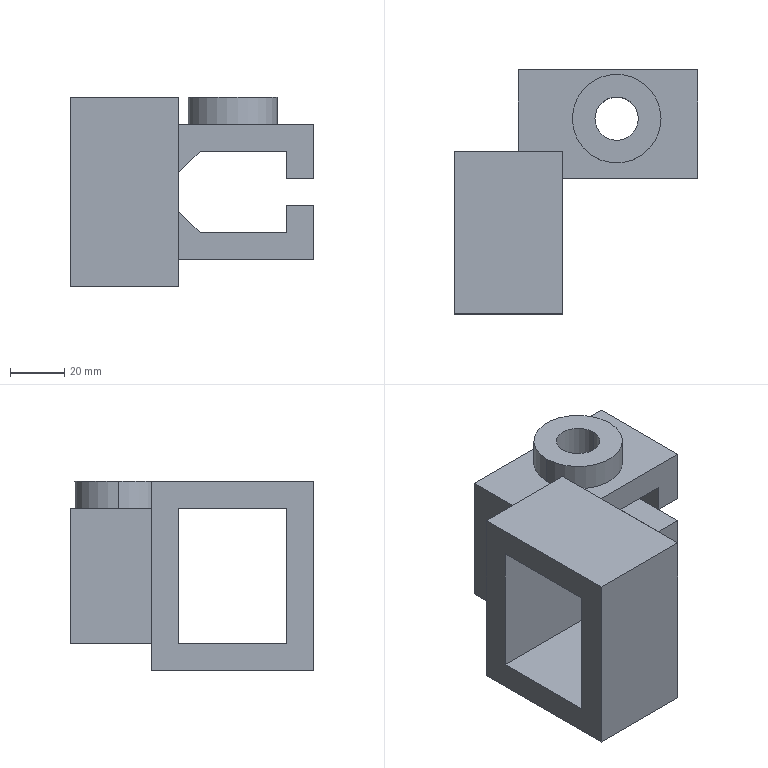Part | SolidWorks | features ICE 5, Extrusion 1 | 1 solid | 32 faces | box 90 x 90 x 70 mm | volume 165265 mm3 | plane 26 | cylinder 6 | commonest cylinder face diameters 16 x4 32.716 x2
STEP:
#1=CARTESIAN_POINT('',(56.358,22.,35.));
#2=VERTEX_POINT('',#1);
#3=CARTESIAN_POINT('',(23.642,22.,35.));
#4=VERTEX_POINT('',#3);
#5=CARTESIAN_POINT('',(40.,22.,35.));
#6=DIRECTION('',(0.,0.,1.));
#7=DIRECTION('',(1.,0.,0.));
#8=AXIS2_PLACEMENT_3D('',#5,#6,#7);
#9=CIRCLE('',#8,16.358);
#10=EDGE_CURVE('',#2,#4,#9,.T.);
#11=ORIENTED_EDGE('',*,*,#10,.F.);
#12=CARTESIAN_POINT('',(56.358,22.,25.));
#13=VERTEX_POINT('',#12);
#14=CARTESIAN_POINT('',(56.358,22.,35.));
#15=DIRECTION('',(0.,0.,-1.));
#16=VECTOR('',#15,1000.);
#17=LINE('',#14,#16);
#18=EDGE_CURVE('',#2,#13,#17,.T.);
#19=ORIENTED_EDGE('',*,*,#18,.T.);
#20=CARTESIAN_POINT('',(23.642,22.,25.));
#21=VERTEX_POINT('',#20);
#22=CARTESIAN_POINT('',(40.,22.,25.));
#23=DIRECTION('',(0.,0.,1.));
#24=DIRECTION('',(-1.,0.,0.));
#25=AXIS2_PLACEMENT_3D('',#22,#23,#24);
#26=CIRCLE('',#25,16.358);
#27=EDGE_CURVE('',#13,#21,#26,.T.);
#28=ORIENTED_EDGE('',*,*,#27,.T.);
#29=CARTESIAN_POINT('',(23.642,22.,35.));
#30=DIRECTION('',(0.,0.,-1.));
#31=VECTOR('',#30,1000.);
#32=LINE('',#29,#31);
#33=EDGE_CURVE('',#4,#21,#32,.T.);
#34=ORIENTED_EDGE('',*,*,#33,.F.);
#35=EDGE_LOOP('',(#11,#19,#28,#34));
#36=FACE_OUTER_BOUND('',#35,.T.);
#37=CARTESIAN_POINT('',(40.,22.,35.));
#38=DIRECTION('',(0.,0.,-1.));
#39=DIRECTION('',(-1.,0.,0.));
#40=AXIS2_PLACEMENT_3D('',#37,#38,#39);
#41=CYLINDRICAL_SURFACE('',#40,16.358);
#42=ADVANCED_FACE('',(#36),#41,.T.);
#43=CARTESIAN_POINT('',(32.,22.,-15.));
#44=VERTEX_POINT('',#43);
#45=CARTESIAN_POINT('',(48.,22.,-15.));
#46=VERTEX_POINT('',#45);
#47=CARTESIAN_POINT('',(40.,22.,-15.));
#48=DIRECTION('',(0.,0.,1.));
#49=DIRECTION('',(1.,0.,0.));
#50=AXIS2_PLACEMENT_3D('',#47,#48,#49);
#51=CIRCLE('',#50,8.);
#52=EDGE_CURVE('',#44,#46,#51,.T.);
#53=ORIENTED_EDGE('',*,*,#52,.T.);
#54=CARTESIAN_POINT('',(48.,22.,-25.));
#55=VERTEX_POINT('',#54);
#56=CARTESIAN_POINT('',(48.,22.,25.));
#57=DIRECTION('',(0.,0.,-1.));
#58=VECTOR('',#57,1000.);
#59=LINE('',#56,#58);
#60=EDGE_CURVE('',#46,#55,#59,.T.);
#61=ORIENTED_EDGE('',*,*,#60,.T.);
#62=CARTESIAN_POINT('',(32.,22.,-25.));
#63=VERTEX_POINT('',#62);
#64=CARTESIAN_POINT('',(40.,22.,-25.));
#65=DIRECTION('',(0.,0.,-1.));
#66=DIRECTION('',(-1.,0.,0.));
#67=AXIS2_PLACEMENT_3D('',#64,#65,#66);
#68=CIRCLE('',#67,8.);
#69=EDGE_CURVE('',#55,#63,#68,.T.);
#70=ORIENTED_EDGE('',*,*,#69,.T.);
#71=CARTESIAN_POINT('',(32.,22.,25.));
#72=DIRECTION('',(0.,0.,-1.));
#73=VECTOR('',#72,1000.);
#74=LINE('',#71,#73);
#75=EDGE_CURVE('',#44,#63,#74,.T.);
#76=ORIENTED_EDGE('',*,*,#75,.F.);
#77=EDGE_LOOP('',(#53,#61,#70,#76));
#78=FACE_OUTER_BOUND('',#77,.T.);
#79=CARTESIAN_POINT('',(40.,22.,25.));
#80=DIRECTION('',(0.,0.,-1.));
#81=DIRECTION('',(-1.,0.,0.));
#82=AXIS2_PLACEMENT_3D('',#79,#80,#81);
#83=CYLINDRICAL_SURFACE('',#82,8.);
#84=ADVANCED_FACE('',(#78),#83,.F.);
#85=CARTESIAN_POINT('',(32.,22.,35.));
#86=VERTEX_POINT('',#85);
#87=CARTESIAN_POINT('',(48.,22.,35.));
#88=VERTEX_POINT('',#87);
#89=CARTESIAN_POINT('',(40.,22.,35.));
#90=DIRECTION('',(0.,0.,1.));
#91=DIRECTION('',(1.,0.,0.));
#92=AXIS2_PLACEMENT_3D('',#89,#90,#91);
#93=CIRCLE('',#92,8.);
#94=EDGE_CURVE('',#86,#88,#93,.T.);
#95=ORIENTED_EDGE('',*,*,#94,.T.);
#96=CARTESIAN_POINT('',(48.,22.,15.));
#97=VERTEX_POINT('',#96);
#98=CARTESIAN_POINT('',(48.,22.,25.));
#99=DIRECTION('',(0.,0.,-1.));
#100=VECTOR('',#99,1000.);
#101=LINE('',#98,#100);
#102=EDGE_CURVE('',#88,#97,#101,.T.);
#103=ORIENTED_EDGE('',*,*,#102,.T.);
#104=CARTESIAN_POINT('',(32.,22.,15.));
#105=VERTEX_POINT('',#104);
#106=CARTESIAN_POINT('',(40.,22.,15.));
#107=DIRECTION('',(0.,0.,-1.));
#108=DIRECTION('',(-1.,0.,0.));
#109=AXIS2_PLACEMENT_3D('',#106,#107,#108);
#110=CIRCLE('',#109,8.);
#111=EDGE_CURVE('',#97,#105,#110,.T.);
#112=ORIENTED_EDGE('',*,*,#111,.T.);
#113=CARTESIAN_POINT('',(32.,22.,25.));
#114=DIRECTION('',(0.,0.,-1.));
#115=VECTOR('',#114,1000.);
#116=LINE('',#113,#115);
#117=EDGE_CURVE('',#86,#105,#116,.T.);
#118=ORIENTED_EDGE('',*,*,#117,.F.);
#119=EDGE_LOOP('',(#95,#103,#112,#118));
#120=FACE_OUTER_BOUND('',#119,.T.);
#121=CARTESIAN_POINT('',(40.,22.,25.));
#122=DIRECTION('',(0.,0.,-1.));
#123=DIRECTION('',(-1.,0.,0.));
#124=AXIS2_PLACEMENT_3D('',#121,#122,#123);
#125=CYLINDRICAL_SURFACE('',#124,8.);
#126=ADVANCED_FACE('',(#120),#125,.F.);
#127=CARTESIAN_POINT('',(20.,0.,25.));
#128=VERTEX_POINT('',#127);
#129=CARTESIAN_POINT('',(20.,10.,25.));
#130=VERTEX_POINT('',#129);
#131=CARTESIAN_POINT('',(20.,-40.,25.));
#132=DIRECTION('',(0.,1.,0.));
#133=VECTOR('',#132,1000.);
#134=LINE('',#131,#133);
#135=EDGE_CURVE('',#128,#130,#134,.T.);
#136=ORIENTED_EDGE('',*,*,#135,.F.);
#137=CARTESIAN_POINT('',(70.,0.,25.));
#138=VERTEX_POINT('',#137);
#139=CARTESIAN_POINT('',(-20.,0.,25.));
#140=DIRECTION('',(1.,0.,0.));
#141=VECTOR('',#140,1000.);
#142=LINE('',#139,#141);
#143=EDGE_CURVE('',#128,#138,#142,.T.);
#144=ORIENTED_EDGE('',*,*,#143,.T.);
#145=CARTESIAN_POINT('',(70.,40.,25.));
#146=VERTEX_POINT('',#145);
#147=CARTESIAN_POINT('',(70.,0.,25.));
#148=DIRECTION('',(0.,1.,0.));
#149=VECTOR('',#148,1000.);
#150=LINE('',#147,#149);
#151=EDGE_CURVE('',#138,#146,#150,.T.);
#152=ORIENTED_EDGE('',*,*,#151,.T.);
#153=CARTESIAN_POINT('',(3.78,40.,25.));
#154=VERTEX_POINT('',#153);
#155=CARTESIAN_POINT('',(3.78,40.,25.));
#156=DIRECTION('',(1.,0.,0.));
#157=VECTOR('',#156,1000.);
#158=LINE('',#155,#157);
#159=EDGE_CURVE('',#154,#146,#158,.T.);
#160=ORIENTED_EDGE('',*,*,#159,.F.);
#161=CARTESIAN_POINT('',(3.78,10.,25.));
#162=VERTEX_POINT('',#161);
#163=CARTESIAN_POINT('',(3.78,40.,25.));
#164=DIRECTION('',(0.,-1.,0.));
#165=VECTOR('',#164,1000.);
#166=LINE('',#163,#165);
#167=EDGE_CURVE('',#154,#162,#166,.T.);
#168=ORIENTED_EDGE('',*,*,#167,.T.);
#169=CARTESIAN_POINT('',(3.78,10.,25.));
#170=DIRECTION('',(1.,0.,0.));
#171=VECTOR('',#170,1000.);
#172=LINE('',#169,#171);
#173=EDGE_CURVE('',#162,#130,#172,.T.);
#174=ORIENTED_EDGE('',*,*,#173,.T.);
#175=EDGE_LOOP('',(#136,#144,#152,#160,#168,#174));
#176=FACE_OUTER_BOUND('',#175,.T.);
#177=CARTESIAN_POINT('',(40.,22.,25.));
#178=DIRECTION('',(0.,0.,1.));
#179=DIRECTION('',(-1.,0.,0.));
#180=AXIS2_PLACEMENT_3D('',#177,#178,#179);
#181=CIRCLE('',#180,16.358);
#182=EDGE_CURVE('',#21,#13,#181,.T.);
#183=ORIENTED_EDGE('',*,*,#182,.F.);
#184=ORIENTED_EDGE('',*,*,#27,.F.);
#185=EDGE_LOOP('',(#183,#184));
#186=FACE_BOUND('',#185,.T.);
#187=CARTESIAN_POINT('',(-20.,10.,25.));
#188=DIRECTION('',(0.,0.,-1.));
#189=DIRECTION('',(-1.,0.,0.));
#190=AXIS2_PLACEMENT_3D('',#187,#188,#189);
#191=PLANE('',#190);
#192=ADVANCED_FACE('',(#176,#186),#191,.F.);
#193=CARTESIAN_POINT('',(40.,22.,-25.));
#194=DIRECTION('',(0.,0.,-1.));
#195=DIRECTION('',(-1.,0.,0.));
#196=AXIS2_PLACEMENT_3D('',#193,#194,#195);
#197=CIRCLE('',#196,8.);
#198=EDGE_CURVE('',#63,#55,#197,.T.);
#199=ORIENTED_EDGE('',*,*,#198,.F.);
#200=ORIENTED_EDGE('',*,*,#69,.F.);
#201=EDGE_LOOP('',(#199,#200));
#202=FACE_BOUND('',#201,.T.);
#203=CARTESIAN_POINT('',(20.,10.,-25.));
#204=VERTEX_POINT('',#203);
#205=CARTESIAN_POINT('',(20.,0.,-25.));
#206=VERTEX_POINT('',#205);
#207=CARTESIAN_POINT('',(20.,0.,-25.));
#208=DIRECTION('',(0.,-1.,0.));
#209=VECTOR('',#208,1000.);
#210=LINE('',#207,#209);
#211=EDGE_CURVE('',#204,#206,#210,.T.);
#212=ORIENTED_EDGE('',*,*,#211,.F.);
#213=CARTESIAN_POINT('',(3.78,10.,-25.));
#214=VERTEX_POINT('',#213);
#215=CARTESIAN_POINT('',(70.,10.,-25.));
#216=DIRECTION('',(-1.,0.,0.));
#217=VECTOR('',#216,1000.);
#218=LINE('',#215,#217);
#219=EDGE_CURVE('',#204,#214,#218,.T.);
#220=ORIENTED_EDGE('',*,*,#219,.T.);
#221=CARTESIAN_POINT('',(3.78,40.,-25.));
#222=VERTEX_POINT('',#221);
#223=CARTESIAN_POINT('',(3.78,40.,-25.));
#224=DIRECTION('',(0.,-1.,0.));
#225=VECTOR('',#224,1000.);
#226=LINE('',#223,#225);
#227=EDGE_CURVE('',#222,#214,#226,.T.);
#228=ORIENTED_EDGE('',*,*,#227,.F.);
#229=CARTESIAN_POINT('',(70.,40.,-25.));
#230=VERTEX_POINT('',#229);
#231=CARTESIAN_POINT('',(70.,40.,-25.));
#232=DIRECTION('',(-1.,0.,0.));
#233=VECTOR('',#232,1000.);
#234=LINE('',#231,#233);
#235=EDGE_CURVE('',#230,#222,#234,.T.);
#236=ORIENTED_EDGE('',*,*,#235,.F.);
#237=CARTESIAN_POINT('',(70.,0.,-25.));
#238=VERTEX_POINT('',#237);
#239=CARTESIAN_POINT('',(70.,0.,-25.));
#240=DIRECTION('',(0.,1.,0.));
#241=VECTOR('',#240,1000.);
#242=LINE('',#239,#241);
#243=EDGE_CURVE('',#238,#230,#242,.T.);
#244=ORIENTED_EDGE('',*,*,#243,.F.);
#245=CARTESIAN_POINT('',(-20.,0.,-25.));
#246=DIRECTION('',(-1.,0.,0.));
#247=VECTOR('',#246,1000.);
#248=LINE('',#245,#247);
#249=EDGE_CURVE('',#238,#206,#248,.T.);
#250=ORIENTED_EDGE('',*,*,#249,.T.);
#251=EDGE_LOOP('',(#212,#220,#228,#236,#244,#250));
#252=FACE_OUTER_BOUND('',#251,.T.);
#253=CARTESIAN_POINT('',(-20.,10.,-25.));
#254=DIRECTION('',(0.,0.,1.));
#255=DIRECTION('',(1.,0.,0.));
#256=AXIS2_PLACEMENT_3D('',#253,#254,#255);
#257=PLANE('',#256);
#258=ADVANCED_FACE('',(#202,#252),#257,.F.);
#259=CARTESIAN_POINT('',(20.,0.,7.));
#260=VERTEX_POINT('',#259);
#261=CARTESIAN_POINT('',(20.,40.,7.));
#262=VERTEX_POINT('',#261);
#263=CARTESIAN_POINT('',(20.,0.,7.));
#264=DIRECTION('',(0.,1.,0.));
#265=VECTOR('',#264,1000.);
#266=LINE('',#263,#265);
#267=EDGE_CURVE('',#260,#262,#266,.T.);
#268=ORIENTED_EDGE('',*,*,#267,.F.);
#269=CARTESIAN_POINT('',(20.,0.,-7.));
#270=VERTEX_POINT('',#269);
#271=CARTESIAN_POINT('',(20.,0.,-25.));
#272=DIRECTION('',(0.,0.,-1.));
#273=VECTOR('',#272,1000.);
#274=LINE('',#271,#273);
#275=EDGE_CURVE('',#260,#270,#274,.T.);
#276=ORIENTED_EDGE('',*,*,#275,.T.);
#277=CARTESIAN_POINT('',(20.,40.,-7.));
#278=VERTEX_POINT('',#277);
#279=CARTESIAN_POINT('',(20.,0.,-7.));
#280=DIRECTION('',(0.,1.,0.));
#281=VECTOR('',#280,1000.);
#282=LINE('',#279,#281);
#283=EDGE_CURVE('',#270,#278,#282,.T.);
#284=ORIENTED_EDGE('',*,*,#283,.T.);
#285=CARTESIAN_POINT('',(20.,40.,7.));
#286=DIRECTION('',(0.,0.,-1.));
#287=VECTOR('',#286,1000.);
#288=LINE('',#285,#287);
#289=EDGE_CURVE('',#262,#278,#288,.T.);
#290=ORIENTED_EDGE('',*,*,#289,.F.);
#291=EDGE_LOOP('',(#268,#276,#284,#290));
#292=FACE_OUTER_BOUND('',#291,.T.);
#293=CARTESIAN_POINT('',(20.,10.,-25.));
#294=DIRECTION('',(-1.,0.,0.));
#295=DIRECTION('',(0.,0.,1.));
#296=AXIS2_PLACEMENT_3D('',#293,#294,#295);
#297=PLANE('',#296);
#298=ADVANCED_FACE('',(#292),#297,.F.);
#299=CARTESIAN_POINT('',(-20.,-40.,-25.));
#300=VERTEX_POINT('',#299);
#301=CARTESIAN_POINT('',(-20.,0.,-25.));
#302=VERTEX_POINT('',#301);
#303=CARTESIAN_POINT('',(-20.,0.,-25.));
#304=DIRECTION('',(0.,1.,0.));
#305=VECTOR('',#304,1000.);
#306=LINE('',#303,#305);
#307=EDGE_CURVE('',#300,#302,#306,.T.);
#308=ORIENTED_EDGE('',*,*,#307,.T.);
#309=CARTESIAN_POINT('',(-20.,0.,25.));
#310=VERTEX_POINT('',#309);
#311=CARTESIAN_POINT('',(-20.,0.,-25.));
#312=DIRECTION('',(0.,0.,1.));
#313=VECTOR('',#312,1000.);
#314=LINE('',#311,#313);
#315=EDGE_CURVE('',#302,#310,#314,.T.);
#316=ORIENTED_EDGE('',*,*,#315,.T.);
#317=CARTESIAN_POINT('',(-20.,-40.,25.));
#318=VERTEX_POINT('',#317);
#319=CARTESIAN_POINT('',(-20.,-40.,25.));
#320=DIRECTION('',(0.,-1.,0.));
#321=VECTOR('',#320,1000.);
#322=LINE('',#319,#321);
#323=EDGE_CURVE('',#310,#318,#322,.T.);
#324=ORIENTED_EDGE('',*,*,#323,.T.);
#325=CARTESIAN_POINT('',(-20.,-40.,-25.));
#326=DIRECTION('',(0.,0.,-1.));
#327=VECTOR('',#326,1000.);
#328=LINE('',#325,#327);
#329=EDGE_CURVE('',#318,#300,#328,.T.);
#330=ORIENTED_EDGE('',*,*,#329,.T.);
#331=EDGE_LOOP('',(#308,#316,#324,#330));
#332=FACE_BOUND('',#331,.T.);
#333=CARTESIAN_POINT('',(-20.,10.,-35.));
#334=VERTEX_POINT('',#333);
#335=CARTESIAN_POINT('',(-20.,10.,35.));
#336=VERTEX_POINT('',#335);
#337=CARTESIAN_POINT('',(-20.,10.,-25.));
#338=DIRECTION('',(0.,0.,1.));
#339=VECTOR('',#338,1000.);
#340=LINE('',#337,#339);
#341=EDGE_CURVE('',#334,#336,#340,.T.);
#342=ORIENTED_EDGE('',*,*,#341,.F.);
#343=CARTESIAN_POINT('',(-20.,-50.,-35.));
#344=VERTEX_POINT('',#343);
#345=CARTESIAN_POINT('',(-20.,10.,-35.));
#346=DIRECTION('',(0.,-1.,0.));
#347=VECTOR('',#346,1000.);
#348=LINE('',#345,#347);
#349=EDGE_CURVE('',#334,#344,#348,.T.);
#350=ORIENTED_EDGE('',*,*,#349,.T.);
#351=CARTESIAN_POINT('',(-20.,-50.,35.));
#352=VERTEX_POINT('',#351);
#353=CARTESIAN_POINT('',(-20.,-50.,-35.));
#354=DIRECTION('',(0.,0.,1.));
#355=VECTOR('',#354,1000.);
#356=LINE('',#353,#355);
#357=EDGE_CURVE('',#344,#352,#356,.T.);
#358=ORIENTED_EDGE('',*,*,#357,.T.);
#359=CARTESIAN_POINT('',(-20.,-50.,35.));
#360=DIRECTION('',(0.,1.,0.));
#361=VECTOR('',#360,1000.);
#362=LINE('',#359,#361);
#363=EDGE_CURVE('',#352,#336,#362,.T.);
#364=ORIENTED_EDGE('',*,*,#363,.T.);
#365=EDGE_LOOP('',(#342,#350,#358,#364));
#366=FACE_OUTER_BOUND('',#365,.T.);
#367=CARTESIAN_POINT('',(-20.,10.,-25.));
#368=DIRECTION('',(1.,0.,0.));
#369=DIRECTION('',(0.,0.,-1.));
#370=AXIS2_PLACEMENT_3D('',#367,#368,#369);
#371=PLANE('',#370);
#372=ADVANCED_FACE('',(#332,#366),#371,.F.);
#373=ORIENTED_EDGE('',*,*,#173,.F.);
#374=CARTESIAN_POINT('',(3.78,10.,-25.));
#375=DIRECTION('',(0.,0.,1.));
#376=VECTOR('',#375,1000.);
#377=LINE('',#374,#376);
#378=EDGE_CURVE('',#214,#162,#377,.T.);
#379=ORIENTED_EDGE('',*,*,#378,.F.);
#380=ORIENTED_EDGE('',*,*,#219,.F.);
#381=CARTESIAN_POINT('',(20.,10.,-35.));
#382=VERTEX_POINT('',#381);
#383=CARTESIAN_POINT('',(20.,10.,-25.));
#384=DIRECTION('',(0.,0.,1.));
#385=VECTOR('',#384,1000.);
#386=LINE('',#383,#385);
#387=EDGE_CURVE('',#382,#204,#386,.T.);
#388=ORIENTED_EDGE('',*,*,#387,.F.);
#389=CARTESIAN_POINT('',(112.195,10.,-35.));
#390=DIRECTION('',(-1.,0.,0.));
#391=VECTOR('',#390,1000.);
#392=LINE('',#389,#391);
#393=EDGE_CURVE('',#382,#334,#392,.T.);
#394=ORIENTED_EDGE('',*,*,#393,.T.);
#395=ORIENTED_EDGE('',*,*,#341,.T.);
#396=CARTESIAN_POINT('',(20.,10.,35.));
#397=VERTEX_POINT('',#396);
#398=CARTESIAN_POINT('',(112.195,10.,35.));
#399=DIRECTION('',(-1.,0.,0.));
#400=VECTOR('',#399,1000.);
#401=LINE('',#398,#400);
#402=EDGE_CURVE('',#397,#336,#401,.T.);
#403=ORIENTED_EDGE('',*,*,#402,.F.);
#404=CARTESIAN_POINT('',(20.,10.,35.));
#405=DIRECTION('',(0.,0.,1.));
#406=VECTOR('',#405,1000.);
#407=LINE('',#404,#406);
#408=EDGE_CURVE('',#130,#397,#407,.T.);
#409=ORIENTED_EDGE('',*,*,#408,.F.);
#410=EDGE_LOOP('',(#373,#379,#380,#388,#394,#395,#403,#409));
#411=FACE_OUTER_BOUND('',#410,.T.);
#412=CARTESIAN_POINT('',(0.,10.,0.));
#413=DIRECTION('',(0.,1.,0.));
#414=DIRECTION('',(0.,0.,1.));
#415=AXIS2_PLACEMENT_3D('',#412,#413,#414);
#416=PLANE('',#415);
#417=ADVANCED_FACE('',(#411),#416,.T.);
#418=ORIENTED_EDGE('',*,*,#275,.F.);
#419=CARTESIAN_POINT('',(28.,0.,15.));
#420=VERTEX_POINT('',#419);
#421=CARTESIAN_POINT('',(28.,0.,15.));
#422=DIRECTION('',(-0.7071,0.,-0.7071));
#423=VECTOR('',#422,1000.);
#424=LINE('',#421,#423);
#425=EDGE_CURVE('',#420,#260,#424,.T.);
#426=ORIENTED_EDGE('',*,*,#425,.F.);
#427=CARTESIAN_POINT('',(60.,0.,15.));
#428=VERTEX_POINT('',#427);
#429=CARTESIAN_POINT('',(28.,0.,15.));
#430=DIRECTION('',(-1.,0.,0.));
#431=VECTOR('',#430,1000.);
#432=LINE('',#429,#431);
#433=EDGE_CURVE('',#428,#420,#432,.T.);
#434=ORIENTED_EDGE('',*,*,#433,.F.);
#435=CARTESIAN_POINT('',(60.,0.,5.));
#436=VERTEX_POINT('',#435);
#437=CARTESIAN_POINT('',(60.,0.,15.));
#438=DIRECTION('',(0.,0.,1.));
#439=VECTOR('',#438,1000.);
#440=LINE('',#437,#439);
#441=EDGE_CURVE('',#436,#428,#440,.T.);
#442=ORIENTED_EDGE('',*,*,#441,.F.);
#443=CARTESIAN_POINT('',(70.,0.,5.));
#444=VERTEX_POINT('',#443);
#445=CARTESIAN_POINT('',(60.,0.,5.));
#446=DIRECTION('',(-1.,0.,0.));
#447=VECTOR('',#446,1000.);
#448=LINE('',#445,#447);
#449=EDGE_CURVE('',#444,#436,#448,.T.);
#450=ORIENTED_EDGE('',*,*,#449,.F.);
#451=CARTESIAN_POINT('',(70.,0.,5.));
#452=DIRECTION('',(0.,0.,-1.));
#453=VECTOR('',#452,1000.);
#454=LINE('',#451,#453);
#455=EDGE_CURVE('',#138,#444,#454,.T.);
#456=ORIENTED_EDGE('',*,*,#455,.F.);
#457=ORIENTED_EDGE('',*,*,#143,.F.);
#458=CARTESIAN_POINT('',(-20.,0.,25.));
#459=DIRECTION('',(1.,0.,0.));
#460=VECTOR('',#459,1000.);
#461=LINE('',#458,#460);
#462=EDGE_CURVE('',#310,#128,#461,.T.);
#463=ORIENTED_EDGE('',*,*,#462,.F.);
#464=ORIENTED_EDGE('',*,*,#315,.F.);
#465=CARTESIAN_POINT('',(-20.,0.,-25.));
#466=DIRECTION('',(-1.,0.,0.));
#467=VECTOR('',#466,1000.);
#468=LINE('',#465,#467);
#469=EDGE_CURVE('',#206,#302,#468,.T.);
#470=ORIENTED_EDGE('',*,*,#469,.F.);
#471=ORIENTED_EDGE('',*,*,#249,.F.);
#472=CARTESIAN_POINT('',(70.,0.,-5.));
#473=VERTEX_POINT('',#472);
#474=CARTESIAN_POINT('',(70.,0.,-25.));
#475=DIRECTION('',(0.,0.,-1.));
#476=VECTOR('',#475,1000.);
#477=LINE('',#474,#476);
#478=EDGE_CURVE('',#473,#238,#477,.T.);
#479=ORIENTED_EDGE('',*,*,#478,.F.);
#480=CARTESIAN_POINT('',(60.,0.,-5.));
#481=VERTEX_POINT('',#480);
#482=CARTESIAN_POINT('',(70.,0.,-5.));
#483=DIRECTION('',(1.,0.,0.));
#484=VECTOR('',#483,1000.);
#485=LINE('',#482,#484);
#486=EDGE_CURVE('',#481,#473,#485,.T.);
#487=ORIENTED_EDGE('',*,*,#486,.F.);
#488=CARTESIAN_POINT('',(60.,0.,-15.));
#489=VERTEX_POINT('',#488);
#490=CARTESIAN_POINT('',(60.,0.,-5.));
#491=DIRECTION('',(0.,0.,1.));
#492=VECTOR('',#491,1000.);
#493=LINE('',#490,#492);
#494=EDGE_CURVE('',#489,#481,#493,.T.);
#495=ORIENTED_EDGE('',*,*,#494,.F.);
#496=CARTESIAN_POINT('',(28.,0.,-15.));
#497=VERTEX_POINT('',#496);
#498=CARTESIAN_POINT('',(60.,0.,-15.));
#499=DIRECTION('',(1.,0.,0.));
#500=VECTOR('',#499,1000.);
#501=LINE('',#498,#500);
#502=EDGE_CURVE('',#497,#489,#501,.T.);
#503=ORIENTED_EDGE('',*,*,#502,.F.);
#504=CARTESIAN_POINT('',(28.,0.,-15.));
#505=DIRECTION('',(0.7071,0.,-0.7071));
#506=VECTOR('',#505,1000.);
#507=LINE('',#504,#506);
#508=EDGE_CURVE('',#270,#497,#507,.T.);
#509=ORIENTED_EDGE('',*,*,#508,.F.);
#510=EDGE_LOOP('',(#418,#426,#434,#442,#450,#456,#457,#463,#464,#470,#471,#479,#487,#495,#503,#509));
#511=FACE_OUTER_BOUND('',#510,.T.);
#512=CARTESIAN_POINT('',(0.,0.,0.));
#513=DIRECTION('',(0.,1.,0.));
#514=DIRECTION('',(0.,0.,1.));
#515=AXIS2_PLACEMENT_3D('',#512,#513,#514);
#516=PLANE('',#515);
#517=ADVANCED_FACE('',(#511),#516,.F.);
#518=ORIENTED_EDGE('',*,*,#243,.T.);
#519=CARTESIAN_POINT('',(70.,40.,-5.));
#520=VERTEX_POINT('',#519);
#521=CARTESIAN_POINT('',(70.,40.,-5.));
#522=DIRECTION('',(0.,0.,-1.));
#523=VECTOR('',#522,1000.);
#524=LINE('',#521,#523);
#525=EDGE_CURVE('',#520,#230,#524,.T.);
#526=ORIENTED_EDGE('',*,*,#525,.F.);
#527=CARTESIAN_POINT('',(70.,0.,-5.));
#528=DIRECTION('',(0.,1.,0.));
#529=VECTOR('',#528,1000.);
#530=LINE('',#527,#529);
#531=EDGE_CURVE('',#473,#520,#530,.T.);
#532=ORIENTED_EDGE('',*,*,#531,.F.);
#533=ORIENTED_EDGE('',*,*,#478,.T.);
#534=EDGE_LOOP('',(#518,#526,#532,#533));
#535=FACE_OUTER_BOUND('',#534,.T.);
#536=CARTESIAN_POINT('',(70.,0.,-25.));
#537=DIRECTION('',(1.,0.,0.));
#538=DIRECTION('',(0.,0.,-1.));
#539=AXIS2_PLACEMENT_3D('',#536,#537,#538);
#540=PLANE('',#539);
#541=ADVANCED_FACE('',(#535),#540,.T.);
#542=ORIENTED_EDGE('',*,*,#531,.T.);
#543=CARTESIAN_POINT('',(60.,40.,-5.));
#544=VERTEX_POINT('',#543);
#545=CARTESIAN_POINT('',(60.,40.,-5.));
#546=DIRECTION('',(1.,0.,0.));
#547=VECTOR('',#546,1000.);
#548=LINE('',#545,#547);
#549=EDGE_CURVE('',#544,#520,#548,.T.);
#550=ORIENTED_EDGE('',*,*,#549,.F.);
#551=CARTESIAN_POINT('',(60.,0.,-5.));
#552=DIRECTION('',(0.,1.,0.));
#553=VECTOR('',#552,1000.);
#554=LINE('',#551,#553);
#555=EDGE_CURVE('',#481,#544,#554,.T.);
#556=ORIENTED_EDGE('',*,*,#555,.F.);
#557=ORIENTED_EDGE('',*,*,#486,.T.);
#558=EDGE_LOOP('',(#542,#550,#556,#557));
#559=FACE_OUTER_BOUND('',#558,.T.);
#560=CARTESIAN_POINT('',(70.,0.,-5.));
#561=DIRECTION('',(0.,0.,1.));
#562=DIRECTION('',(1.,0.,0.));
#563=AXIS2_PLACEMENT_3D('',#560,#561,#562);
#564=PLANE('',#563);
#565=ADVANCED_FACE('',(#559),#564,.T.);
#566=ORIENTED_EDGE('',*,*,#555,.T.);
#567=CARTESIAN_POINT('',(60.,40.,-15.));
#568=VERTEX_POINT('',#567);
#569=CARTESIAN_POINT('',(60.,40.,-15.));
#570=DIRECTION('',(0.,0.,1.));
#571=VECTOR('',#570,1000.);
#572=LINE('',#569,#571);
#573=EDGE_CURVE('',#568,#544,#572,.T.);
#574=ORIENTED_EDGE('',*,*,#573,.F.);
#575=CARTESIAN_POINT('',(60.,0.,-15.));
#576=DIRECTION('',(0.,1.,0.));
#577=VECTOR('',#576,1000.);
#578=LINE('',#575,#577);
#579=EDGE_CURVE('',#489,#568,#578,.T.);
#580=ORIENTED_EDGE('',*,*,#579,.F.);
#581=ORIENTED_EDGE('',*,*,#494,.T.);
#582=EDGE_LOOP('',(#566,#574,#580,#581));
#583=FACE_OUTER_BOUND('',#582,.T.);
#584=CARTESIAN_POINT('',(60.,0.,-5.));
#585=DIRECTION('',(-1.,0.,0.));
#586=DIRECTION('',(0.,0.,1.));
#587=AXIS2_PLACEMENT_3D('',#584,#585,#586);
#588=PLANE('',#587);
#589=ADVANCED_FACE('',(#583),#588,.T.);
#590=ORIENTED_EDGE('',*,*,#52,.F.);
#591=CARTESIAN_POINT('',(40.,22.,-15.));
#592=DIRECTION('',(0.,0.,1.));
#593=DIRECTION('',(1.,0.,0.));
#594=AXIS2_PLACEMENT_3D('',#591,#592,#593);
#595=CIRCLE('',#594,8.);
#596=EDGE_CURVE('',#46,#44,#595,.T.);
#597=ORIENTED_EDGE('',*,*,#596,.F.);
#598=EDGE_LOOP('',(#590,#597));
#599=FACE_BOUND('',#598,.T.);
#600=ORIENTED_EDGE('',*,*,#579,.T.);
#601=CARTESIAN_POINT('',(28.,40.,-15.));
#602=VERTEX_POINT('',#601);
#603=CARTESIAN_POINT('',(28.,40.,-15.));
#604=DIRECTION('',(1.,0.,0.));
#605=VECTOR('',#604,1000.);
#606=LINE('',#603,#605);
#607=EDGE_CURVE('',#602,#568,#606,.T.);
#608=ORIENTED_EDGE('',*,*,#607,.F.);
#609=CARTESIAN_POINT('',(28.,0.,-15.));
#610=DIRECTION('',(0.,1.,0.));
#611=VECTOR('',#610,1000.);
#612=LINE('',#609,#611);
#613=EDGE_CURVE('',#497,#602,#612,.T.);
#614=ORIENTED_EDGE('',*,*,#613,.F.);
#615=ORIENTED_EDGE('',*,*,#502,.T.);
#616=EDGE_LOOP('',(#600,#608,#614,#615));
#617=FACE_OUTER_BOUND('',#616,.T.);
#618=CARTESIAN_POINT('',(60.,0.,-15.));
#619=DIRECTION('',(0.,0.,1.));
#620=DIRECTION('',(1.,0.,0.));
#621=AXIS2_PLACEMENT_3D('',#618,#619,#620);
#622=PLANE('',#621);
#623=ADVANCED_FACE('',(#599,#617),#622,.T.);
#624=ORIENTED_EDGE('',*,*,#613,.T.);
#625=CARTESIAN_POINT('',(20.,40.,-7.));
#626=DIRECTION('',(0.7071,0.,-0.7071));
#627=VECTOR('',#626,1000.);
#628=LINE('',#625,#627);
#629=EDGE_CURVE('',#278,#602,#628,.T.);
#630=ORIENTED_EDGE('',*,*,#629,.F.);
#631=ORIENTED_EDGE('',*,*,#283,.F.);
#632=ORIENTED_EDGE('',*,*,#508,.T.);
#633=EDGE_LOOP('',(#624,#630,#631,#632));
#634=FACE_OUTER_BOUND('',#633,.T.);
#635=CARTESIAN_POINT('',(28.,0.,-15.));
#636=DIRECTION('',(0.7071,0.,0.7071));
#637=DIRECTION('',(0.7071,0.,-0.7071));
#638=AXIS2_PLACEMENT_3D('',#635,#636,#637);
#639=PLANE('',#638);
#640=ADVANCED_FACE('',(#634),#639,.T.);
#641=ORIENTED_EDGE('',*,*,#267,.T.);
#642=CARTESIAN_POINT('',(28.,40.,15.));
#643=VERTEX_POINT('',#642);
#644=CARTESIAN_POINT('',(28.,40.,15.));
#645=DIRECTION('',(-0.7071,0.,-0.7071));
#646=VECTOR('',#645,1000.);
#647=LINE('',#644,#646);
#648=EDGE_CURVE('',#643,#262,#647,.T.);
#649=ORIENTED_EDGE('',*,*,#648,.F.);
#650=CARTESIAN_POINT('',(28.,0.,15.));
#651=DIRECTION('',(0.,1.,0.));
#652=VECTOR('',#651,1000.);
#653=LINE('',#650,#652);
#654=EDGE_CURVE('',#420,#643,#653,.T.);
#655=ORIENTED_EDGE('',*,*,#654,.F.);
#656=ORIENTED_EDGE('',*,*,#425,.T.);
#657=EDGE_LOOP('',(#641,#649,#655,#656));
#658=FACE_OUTER_BOUND('',#657,.T.);
#659=CARTESIAN_POINT('',(28.,0.,15.));
#660=DIRECTION('',(0.7071,0.,-0.7071));
#661=DIRECTION('',(-0.7071,0.,-0.7071));
#662=AXIS2_PLACEMENT_3D('',#659,#660,#661);
#663=PLANE('',#662);
#664=ADVANCED_FACE('',(#658),#663,.T.);
#665=CARTESIAN_POINT('',(40.,22.,15.));
#666=DIRECTION('',(0.,0.,-1.));
#667=DIRECTION('',(-1.,0.,0.));
#668=AXIS2_PLACEMENT_3D('',#665,#666,#667);
#669=CIRCLE('',#668,8.);
#670=EDGE_CURVE('',#105,#97,#669,.T.);
#671=ORIENTED_EDGE('',*,*,#670,.F.);
#672=ORIENTED_EDGE('',*,*,#111,.F.);
#673=EDGE_LOOP('',(#671,#672));
#674=FACE_BOUND('',#673,.T.);
#675=ORIENTED_EDGE('',*,*,#654,.T.);
#676=CARTESIAN_POINT('',(60.,40.,15.));
#677=VERTEX_POINT('',#676);
#678=CARTESIAN_POINT('',(60.,40.,15.));
#679=DIRECTION('',(-1.,0.,0.));
#680=VECTOR('',#679,1000.);
#681=LINE('',#678,#680);
#682=EDGE_CURVE('',#677,#643,#681,.T.);
#683=ORIENTED_EDGE('',*,*,#682,.F.);
#684=CARTESIAN_POINT('',(60.,0.,15.));
#685=DIRECTION('',(0.,1.,0.));
#686=VECTOR('',#685,1000.);
#687=LINE('',#684,#686);
#688=EDGE_CURVE('',#428,#677,#687,.T.);
#689=ORIENTED_EDGE('',*,*,#688,.F.);
#690=ORIENTED_EDGE('',*,*,#433,.T.);
#691=EDGE_LOOP('',(#675,#683,#689,#690));
#692=FACE_OUTER_BOUND('',#691,.T.);
#693=CARTESIAN_POINT('',(28.,0.,15.));
#694=DIRECTION('',(0.,0.,-1.));
#695=DIRECTION('',(-1.,0.,0.));
#696=AXIS2_PLACEMENT_3D('',#693,#694,#695);
#697=PLANE('',#696);
#698=ADVANCED_FACE('',(#674,#692),#697,.T.);
#699=ORIENTED_EDGE('',*,*,#688,.T.);
#700=CARTESIAN_POINT('',(60.,40.,5.));
#701=VERTEX_POINT('',#700);
#702=CARTESIAN_POINT('',(60.,40.,5.));
#703=DIRECTION('',(0.,0.,1.));
#704=VECTOR('',#703,1000.);
#705=LINE('',#702,#704);
#706=EDGE_CURVE('',#701,#677,#705,.T.);
#707=ORIENTED_EDGE('',*,*,#706,.F.);
#708=CARTESIAN_POINT('',(60.,0.,5.));
#709=DIRECTION('',(0.,1.,0.));
#710=VECTOR('',#709,1000.);
#711=LINE('',#708,#710);
#712=EDGE_CURVE('',#436,#701,#711,.T.);
#713=ORIENTED_EDGE('',*,*,#712,.F.);
#714=ORIENTED_EDGE('',*,*,#441,.T.);
#715=EDGE_LOOP('',(#699,#707,#713,#714));
#716=FACE_OUTER_BOUND('',#715,.T.);
#717=CARTESIAN_POINT('',(60.,0.,15.));
#718=DIRECTION('',(-1.,0.,0.));
#719=DIRECTION('',(0.,0.,1.));
#720=AXIS2_PLACEMENT_3D('',#717,#718,#719);
#721=PLANE('',#720);
#722=ADVANCED_FACE('',(#716),#721,.T.);
#723=ORIENTED_EDGE('',*,*,#712,.T.);
#724=CARTESIAN_POINT('',(70.,40.,5.));
#725=VERTEX_POINT('',#724);
#726=CARTESIAN_POINT('',(70.,40.,5.));
#727=DIRECTION('',(-1.,0.,0.));
#728=VECTOR('',#727,1000.);
#729=LINE('',#726,#728);
#730=EDGE_CURVE('',#725,#701,#729,.T.);
#731=ORIENTED_EDGE('',*,*,#730,.F.);
#732=CARTESIAN_POINT('',(70.,0.,5.));
#733=DIRECTION('',(0.,1.,0.));
#734=VECTOR('',#733,1000.);
#735=LINE('',#732,#734);
#736=EDGE_CURVE('',#444,#725,#735,.T.);
#737=ORIENTED_EDGE('',*,*,#736,.F.);
#738=ORIENTED_EDGE('',*,*,#449,.T.);
#739=EDGE_LOOP('',(#723,#731,#737,#738));
#740=FACE_OUTER_BOUND('',#739,.T.);
#741=CARTESIAN_POINT('',(60.,0.,5.));
#742=DIRECTION('',(0.,0.,-1.));
#743=DIRECTION('',(-1.,0.,0.));
#744=AXIS2_PLACEMENT_3D('',#741,#742,#743);
#745=PLANE('',#744);
#746=ADVANCED_FACE('',(#740),#745,.T.);
#747=ORIENTED_EDGE('',*,*,#736,.T.);
#748=CARTESIAN_POINT('',(70.,40.,25.));
#749=DIRECTION('',(0.,0.,-1.));
#750=VECTOR('',#749,1000.);
#751=LINE('',#748,#750);
#752=EDGE_CURVE('',#146,#725,#751,.T.);
#753=ORIENTED_EDGE('',*,*,#752,.F.);
#754=ORIENTED_EDGE('',*,*,#151,.F.);
#755=ORIENTED_EDGE('',*,*,#455,.T.);
#756=EDGE_LOOP('',(#747,#753,#754,#755));
#757=FACE_OUTER_BOUND('',#756,.T.);
#758=CARTESIAN_POINT('',(70.,0.,5.));
#759=DIRECTION('',(1.,0.,0.));
#760=DIRECTION('',(0.,0.,-1.));
#761=AXIS2_PLACEMENT_3D('',#758,#759,#760);
#762=PLANE('',#761);
#763=ADVANCED_FACE('',(#757),#762,.T.);
#764=ORIENTED_EDGE('',*,*,#469,.T.);
#765=ORIENTED_EDGE('',*,*,#307,.F.);
#766=CARTESIAN_POINT('',(20.,-40.,-25.));
#767=VERTEX_POINT('',#766);
#768=CARTESIAN_POINT('',(112.195,-40.,-25.));
#769=DIRECTION('',(-1.,0.,0.));
#770=VECTOR('',#769,1000.);
#771=LINE('',#768,#770);
#772=EDGE_CURVE('',#767,#300,#771,.T.);
#773=ORIENTED_EDGE('',*,*,#772,.F.);
#774=CARTESIAN_POINT('',(20.,0.,-25.));
#775=DIRECTION('',(0.,-1.,0.));
#776=VECTOR('',#775,1000.);
#777=LINE('',#774,#776);
#778=EDGE_CURVE('',#206,#767,#777,.T.);
#779=ORIENTED_EDGE('',*,*,#778,.F.);
#780=EDGE_LOOP('',(#764,#765,#773,#779));
#781=FACE_OUTER_BOUND('',#780,.T.);
#782=CARTESIAN_POINT('',(112.195,0.,-25.));
#783=DIRECTION('',(0.,0.,1.));
#784=DIRECTION('',(1.,0.,0.));
#785=AXIS2_PLACEMENT_3D('',#782,#783,#784);
#786=PLANE('',#785);
#787=ADVANCED_FACE('',(#781),#786,.T.);
#788=ORIENTED_EDGE('',*,*,#462,.T.);
#789=CARTESIAN_POINT('',(20.,-40.,25.));
#790=VERTEX_POINT('',#789);
#791=CARTESIAN_POINT('',(20.,-40.,25.));
#792=DIRECTION('',(0.,1.,0.));
#793=VECTOR('',#792,1000.);
#794=LINE('',#791,#793);
#795=EDGE_CURVE('',#790,#128,#794,.T.);
#796=ORIENTED_EDGE('',*,*,#795,.F.);
#797=CARTESIAN_POINT('',(112.195,-40.,25.));
#798=DIRECTION('',(-1.,0.,0.));
#799=VECTOR('',#798,1000.);
#800=LINE('',#797,#799);
#801=EDGE_CURVE('',#790,#318,#800,.T.);
#802=ORIENTED_EDGE('',*,*,#801,.T.);
#803=ORIENTED_EDGE('',*,*,#323,.F.);
#804=EDGE_LOOP('',(#788,#796,#802,#803));
#805=FACE_OUTER_BOUND('',#804,.T.);
#806=CARTESIAN_POINT('',(112.195,-40.,25.));
#807=DIRECTION('',(0.,0.,-1.));
#808=DIRECTION('',(-1.,0.,0.));
#809=AXIS2_PLACEMENT_3D('',#806,#807,#808);
#810=PLANE('',#809);
#811=ADVANCED_FACE('',(#805),#810,.T.);
#812=CARTESIAN_POINT('',(20.,-40.,-25.));
#813=DIRECTION('',(0.,0.,1.));
#814=VECTOR('',#813,1000.);
#815=LINE('',#812,#814);
#816=EDGE_CURVE('',#767,#790,#815,.T.);
#817=ORIENTED_EDGE('',*,*,#816,.F.);
#818=ORIENTED_EDGE('',*,*,#772,.T.);
#819=ORIENTED_EDGE('',*,*,#329,.F.);
#820=ORIENTED_EDGE('',*,*,#801,.F.);
#821=EDGE_LOOP('',(#817,#818,#819,#820));
#822=FACE_OUTER_BOUND('',#821,.T.);
#823=CARTESIAN_POINT('',(112.195,-40.,-25.));
#824=DIRECTION('',(0.,1.,0.));
#825=DIRECTION('',(0.,0.,1.));
#826=AXIS2_PLACEMENT_3D('',#823,#824,#825);
#827=PLANE('',#826);
#828=ADVANCED_FACE('',(#822),#827,.T.);
#829=CARTESIAN_POINT('',(20.,-50.,35.));
#830=VERTEX_POINT('',#829);
#831=CARTESIAN_POINT('',(20.,-50.,35.));
#832=DIRECTION('',(0.,-1.,0.));
#833=VECTOR('',#832,1000.);
#834=LINE('',#831,#833);
#835=EDGE_CURVE('',#397,#830,#834,.T.);
#836=ORIENTED_EDGE('',*,*,#835,.F.);
#837=ORIENTED_EDGE('',*,*,#402,.T.);
#838=ORIENTED_EDGE('',*,*,#363,.F.);
#839=CARTESIAN_POINT('',(112.195,-50.,35.));
#840=DIRECTION('',(-1.,0.,0.));
#841=VECTOR('',#840,1000.);
#842=LINE('',#839,#841);
#843=EDGE_CURVE('',#830,#352,#842,.T.);
#844=ORIENTED_EDGE('',*,*,#843,.F.);
#845=EDGE_LOOP('',(#836,#837,#838,#844));
#846=FACE_OUTER_BOUND('',#845,.T.);
#847=CARTESIAN_POINT('',(112.195,-50.,35.));
#848=DIRECTION('',(0.,0.,1.));
#849=DIRECTION('',(1.,0.,0.));
#850=AXIS2_PLACEMENT_3D('',#847,#848,#849);
#851=PLANE('',#850);
#852=ADVANCED_FACE('',(#846),#851,.T.);
#853=CARTESIAN_POINT('',(20.,-50.,-35.));
#854=VERTEX_POINT('',#853);
#855=CARTESIAN_POINT('',(20.,-50.,-35.));
#856=DIRECTION('',(0.,0.,-1.));
#857=VECTOR('',#856,1000.);
#858=LINE('',#855,#857);
#859=EDGE_CURVE('',#830,#854,#858,.T.);
#860=ORIENTED_EDGE('',*,*,#859,.F.);
#861=ORIENTED_EDGE('',*,*,#843,.T.);
#862=ORIENTED_EDGE('',*,*,#357,.F.);
#863=CARTESIAN_POINT('',(112.195,-50.,-35.));
#864=DIRECTION('',(-1.,0.,0.));
#865=VECTOR('',#864,1000.);
#866=LINE('',#863,#865);
#867=EDGE_CURVE('',#854,#344,#866,.T.);
#868=ORIENTED_EDGE('',*,*,#867,.F.);
#869=EDGE_LOOP('',(#860,#861,#862,#868));
#870=FACE_OUTER_BOUND('',#869,.T.);
#871=CARTESIAN_POINT('',(112.195,-50.,-35.));
#872=DIRECTION('',(0.,-1.,0.));
#873=DIRECTION('',(0.,0.,-1.));
#874=AXIS2_PLACEMENT_3D('',#871,#872,#873);
#875=PLANE('',#874);
#876=ADVANCED_FACE('',(#870),#875,.T.);
#877=CARTESIAN_POINT('',(20.,10.,-35.));
#878=DIRECTION('',(0.,1.,0.));
#879=VECTOR('',#878,1000.);
#880=LINE('',#877,#879);
#881=EDGE_CURVE('',#854,#382,#880,.T.);
#882=ORIENTED_EDGE('',*,*,#881,.F.);
#883=ORIENTED_EDGE('',*,*,#867,.T.);
#884=ORIENTED_EDGE('',*,*,#349,.F.);
#885=ORIENTED_EDGE('',*,*,#393,.F.);
#886=EDGE_LOOP('',(#882,#883,#884,#885));
#887=FACE_OUTER_BOUND('',#886,.T.);
#888=CARTESIAN_POINT('',(112.195,10.,-35.));
#889=DIRECTION('',(0.,0.,-1.));
#890=DIRECTION('',(-1.,0.,0.));
#891=AXIS2_PLACEMENT_3D('',#888,#889,#890);
#892=PLANE('',#891);
#893=ADVANCED_FACE('',(#887),#892,.T.);
#894=ORIENTED_EDGE('',*,*,#211,.T.);
#895=ORIENTED_EDGE('',*,*,#778,.T.);
#896=ORIENTED_EDGE('',*,*,#816,.T.);
#897=ORIENTED_EDGE('',*,*,#795,.T.);
#898=ORIENTED_EDGE('',*,*,#135,.T.);
#899=ORIENTED_EDGE('',*,*,#408,.T.);
#900=ORIENTED_EDGE('',*,*,#835,.T.);
#901=ORIENTED_EDGE('',*,*,#859,.T.);
#902=ORIENTED_EDGE('',*,*,#881,.T.);
#903=ORIENTED_EDGE('',*,*,#387,.T.);
#904=EDGE_LOOP('',(#894,#895,#896,#897,#898,#899,#900,#901,#902,#903));
#905=FACE_OUTER_BOUND('',#904,.T.);
#906=CARTESIAN_POINT('',(20.,10.,-25.));
#907=DIRECTION('',(-1.,0.,0.));
#908=DIRECTION('',(0.,0.,1.));
#909=AXIS2_PLACEMENT_3D('',#906,#907,#908);
#910=PLANE('',#909);
#911=ADVANCED_FACE('',(#905),#910,.F.);
#912=ORIENTED_EDGE('',*,*,#378,.T.);
#913=ORIENTED_EDGE('',*,*,#167,.F.);
#914=CARTESIAN_POINT('',(3.78,40.,-25.));
#915=DIRECTION('',(0.,0.,1.));
#916=VECTOR('',#915,1000.);
#917=LINE('',#914,#916);
#918=EDGE_CURVE('',#222,#154,#917,.T.);
#919=ORIENTED_EDGE('',*,*,#918,.F.);
#920=ORIENTED_EDGE('',*,*,#227,.T.);
#921=EDGE_LOOP('',(#912,#913,#919,#920));
#922=FACE_OUTER_BOUND('',#921,.T.);
#923=CARTESIAN_POINT('',(3.78,40.,-25.));
#924=DIRECTION('',(1.,0.,0.));
#925=DIRECTION('',(0.,0.,-1.));
#926=AXIS2_PLACEMENT_3D('',#923,#924,#925);
#927=PLANE('',#926);
#928=ADVANCED_FACE('',(#922),#927,.F.);
#929=ORIENTED_EDGE('',*,*,#289,.T.);
#930=ORIENTED_EDGE('',*,*,#629,.T.);
#931=ORIENTED_EDGE('',*,*,#607,.T.);
#932=ORIENTED_EDGE('',*,*,#573,.T.);
#933=ORIENTED_EDGE('',*,*,#549,.T.);
#934=ORIENTED_EDGE('',*,*,#525,.T.);
#935=ORIENTED_EDGE('',*,*,#235,.T.);
#936=ORIENTED_EDGE('',*,*,#918,.T.);
#937=ORIENTED_EDGE('',*,*,#159,.T.);
#938=ORIENTED_EDGE('',*,*,#752,.T.);
#939=ORIENTED_EDGE('',*,*,#730,.T.);
#940=ORIENTED_EDGE('',*,*,#706,.T.);
#941=ORIENTED_EDGE('',*,*,#682,.T.);
#942=ORIENTED_EDGE('',*,*,#648,.T.);
#943=EDGE_LOOP('',(#929,#930,#931,#932,#933,#934,#935,#936,#937,#938,#939,#940,#941,#942));
#944=FACE_OUTER_BOUND('',#943,.T.);
#945=CARTESIAN_POINT('',(0.,40.,0.));
#946=DIRECTION('',(0.,-1.,0.));
#947=DIRECTION('',(0.,0.,-1.));
#948=AXIS2_PLACEMENT_3D('',#945,#946,#947);
#949=PLANE('',#948);
#950=ADVANCED_FACE('',(#944),#949,.F.);
#951=ORIENTED_EDGE('',*,*,#102,.F.);
#952=CARTESIAN_POINT('',(40.,22.,35.));
#953=DIRECTION('',(0.,0.,1.));
#954=DIRECTION('',(1.,0.,0.));
#955=AXIS2_PLACEMENT_3D('',#952,#953,#954);
#956=CIRCLE('',#955,8.);
#957=EDGE_CURVE('',#88,#86,#956,.T.);
#958=ORIENTED_EDGE('',*,*,#957,.T.);
#959=ORIENTED_EDGE('',*,*,#117,.T.);
#960=ORIENTED_EDGE('',*,*,#670,.T.);
#961=EDGE_LOOP('',(#951,#958,#959,#960));
#962=FACE_OUTER_BOUND('',#961,.T.);
#963=CARTESIAN_POINT('',(40.,22.,25.));
#964=DIRECTION('',(0.,0.,-1.));
#965=DIRECTION('',(-1.,0.,0.));
#966=AXIS2_PLACEMENT_3D('',#963,#964,#965);
#967=CYLINDRICAL_SURFACE('',#966,8.);
#968=ADVANCED_FACE('',(#962),#967,.F.);
#969=ORIENTED_EDGE('',*,*,#60,.F.);
#970=ORIENTED_EDGE('',*,*,#596,.T.);
#971=ORIENTED_EDGE('',*,*,#75,.T.);
#972=ORIENTED_EDGE('',*,*,#198,.T.);
#973=EDGE_LOOP('',(#969,#970,#971,#972));
#974=FACE_OUTER_BOUND('',#973,.T.);
#975=CARTESIAN_POINT('',(40.,22.,25.));
#976=DIRECTION('',(0.,0.,-1.));
#977=DIRECTION('',(-1.,0.,0.));
#978=AXIS2_PLACEMENT_3D('',#975,#976,#977);
#979=CYLINDRICAL_SURFACE('',#978,8.);
#980=ADVANCED_FACE('',(#974),#979,.F.);
#981=CARTESIAN_POINT('',(40.,22.,35.));
#982=DIRECTION('',(0.,0.,1.));
#983=DIRECTION('',(1.,0.,0.));
#984=AXIS2_PLACEMENT_3D('',#981,#982,#983);
#985=CIRCLE('',#984,16.358);
#986=EDGE_CURVE('',#4,#2,#985,.T.);
#987=ORIENTED_EDGE('',*,*,#986,.T.);
#988=ORIENTED_EDGE('',*,*,#10,.T.);
#989=EDGE_LOOP('',(#987,#988));
#990=FACE_OUTER_BOUND('',#989,.T.);
#991=ORIENTED_EDGE('',*,*,#94,.F.);
#992=ORIENTED_EDGE('',*,*,#957,.F.);
#993=EDGE_LOOP('',(#991,#992));
#994=FACE_BOUND('',#993,.T.);
#995=CARTESIAN_POINT('',(40.,22.,35.));
#996=DIRECTION('',(0.,0.,1.));
#997=DIRECTION('',(1.,0.,0.));
#998=AXIS2_PLACEMENT_3D('',#995,#996,#997);
#999=PLANE('',#998);
#1000=ADVANCED_FACE('',(#990,#994),#999,.T.);
#1001=ORIENTED_EDGE('',*,*,#18,.F.);
#1002=ORIENTED_EDGE('',*,*,#986,.F.);
#1003=ORIENTED_EDGE('',*,*,#33,.T.);
#1004=ORIENTED_EDGE('',*,*,#182,.T.);
#1005=EDGE_LOOP('',(#1001,#1002,#1003,#1004));
#1006=FACE_OUTER_BOUND('',#1005,.T.);
#1007=CARTESIAN_POINT('',(40.,22.,35.));
#1008=DIRECTION('',(0.,0.,-1.));
#1009=DIRECTION('',(-1.,0.,0.));
#1010=AXIS2_PLACEMENT_3D('',#1007,#1008,#1009);
#1011=CYLINDRICAL_SURFACE('',#1010,16.358);
#1012=ADVANCED_FACE('',(#1006),#1011,.T.);
#1013=CLOSED_SHELL('',(#42,#84,#126,#192,#258,#298,#372,#417,#517,#541,#565,#589,#623,#640,#664,#698,#722,#746,#763,#787,#811,#828,#852,#876,#893,#911,#928,#950,#968,#980,#1000,#1012));
#1014=MANIFOLD_SOLID_BREP('',#1013);
#1015=CARTESIAN_POINT('',(0.,0.,0.));
#1016=DIRECTION('',(0.,0.,1.));
#1017=DIRECTION('',(1.,0.,0.));
#1018=AXIS2_PLACEMENT_3D('',#1015,#1016,#1017);
#1019=(LENGTH_UNIT()NAMED_UNIT(*)SI_UNIT(.MILLI.,.METRE.));
#1020=UNCERTAINTY_MEASURE_WITH_UNIT(LENGTH_MEASURE(0.00001),#1019,'','');
#1021=(NAMED_UNIT(*)PLANE_ANGLE_UNIT()SI_UNIT($,.RADIAN.));
#1022=(NAMED_UNIT(*)SI_UNIT($,.STERADIAN.)SOLID_ANGLE_UNIT());
#1023=(GEOMETRIC_REPRESENTATION_CONTEXT(3)GLOBAL_UNCERTAINTY_ASSIGNED_CONTEXT((#1020))GLOBAL_UNIT_ASSIGNED_CONTEXT((#1019,#1021,#1022))REPRESENTATION_CONTEXT('',''));
#1024=ADVANCED_BREP_SHAPE_REPRESENTATION('',(#1014,#1018),#1023);